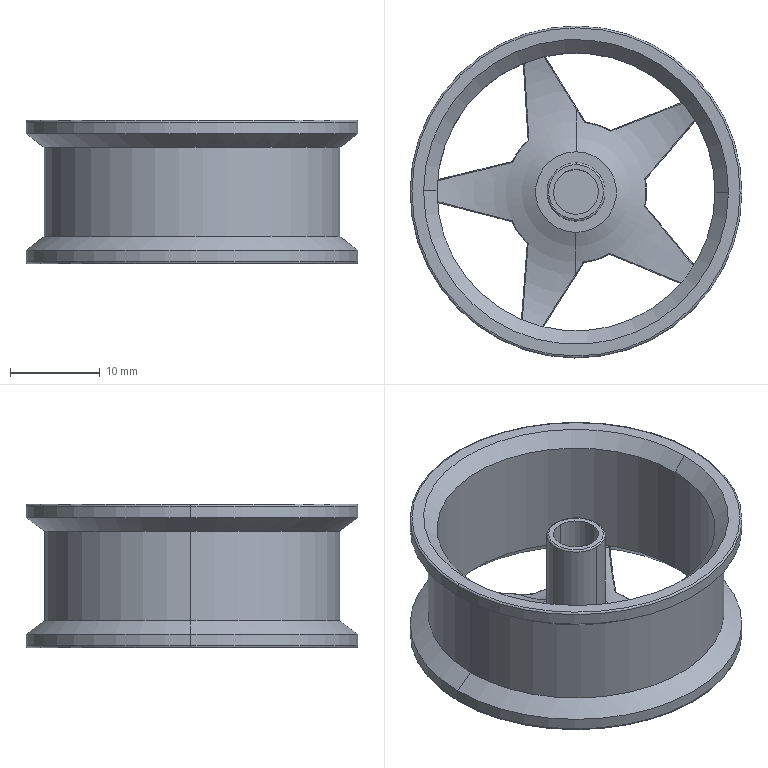Part | SolidWorks | features SplitBody 1 | 1 solid | 130 faces | box 37 x 37 x 16 mm | volume 2778 mm3 | spline 50 | torus 36 | cylinder 19 | plane 17 | cone 8 | commonest cylinder face diameters 15.788 x5 5 x4 37 x4 6.5 x2 31 x2 33 x2